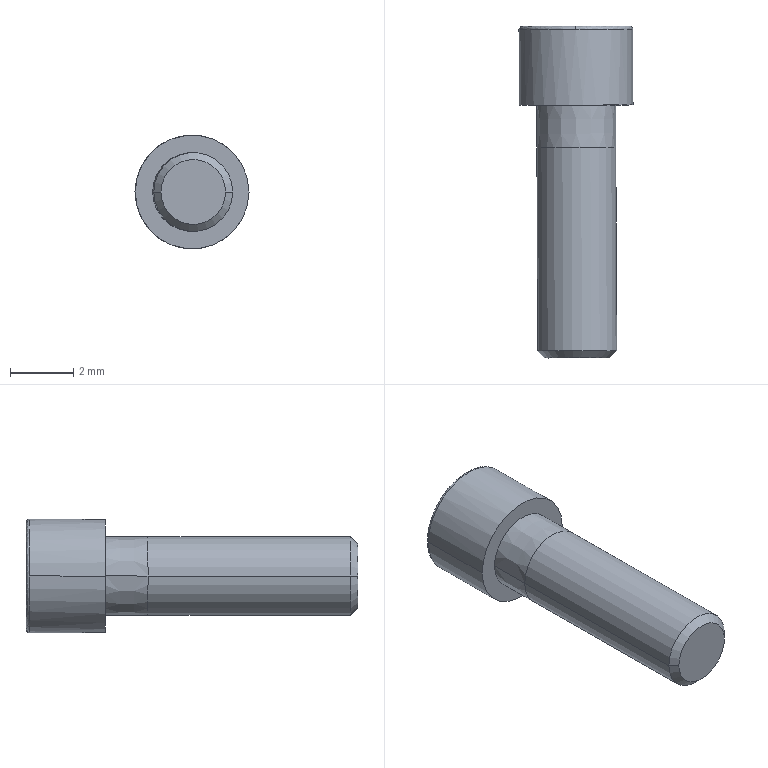Part | SolidWorks | features BaseBody 1 | 1 solid | 20 faces | box 3.61 x 10.512 x 3.6 mm | volume 60.691 mm3 | plane 10 | cylinder 4 | cone 4 | spline 2 | commonest cylinder face diameters 2.5 x2 3.6 x2
STEP:
#1=CARTESIAN_POINT('',(590.444,59.349,88.732));
#2=VERTEX_POINT('',#1);
#3=CARTESIAN_POINT('',(590.444,59.349,92.132));
#4=VERTEX_POINT('',#3);
#5=CARTESIAN_POINT('',(590.444,59.349,88.732));
#6=CARTESIAN_POINT('',(593.844,59.364,88.732));
#7=CARTESIAN_POINT('',(593.844,59.364,92.132));
#8=CARTESIAN_POINT('',(590.444,59.349,92.132));
#9=(BOUNDED_CURVE()B_SPLINE_CURVE(3,(#5,#6,#7,#8),.UNSPECIFIED.,.F.,.F.)B_SPLINE_CURVE_WITH_KNOTS((4,4),(0.,1.),.UNSPECIFIED.)CURVE()GEOMETRIC_REPRESENTATION_ITEM()RATIONAL_B_SPLINE_CURVE((1.,0.3333,0.3333,1.))REPRESENTATION_ITEM(''));
#10=EDGE_CURVE('',#2,#4,#9,.T.);
#11=ORIENTED_EDGE('',*,*,#10,.T.);
#12=CARTESIAN_POINT('',(590.444,59.249,92.232));
#13=VERTEX_POINT('',#12);
#14=CARTESIAN_POINT('',(590.444,59.249,92.132));
#15=DIRECTION('',(1.,0.004352,0.));
#16=DIRECTION('',(0.,0.,1.));
#17=AXIS2_PLACEMENT_3D('',#14,#15,#16);
#18=CIRCLE('',#17,0.1);
#19=EDGE_CURVE('',#4,#13,#18,.T.);
#20=ORIENTED_EDGE('',*,*,#19,.T.);
#21=CARTESIAN_POINT('',(592.244,59.257,90.432));
#22=VERTEX_POINT('',#21);
#23=CARTESIAN_POINT('',(590.444,59.249,90.432));
#24=DIRECTION('',(0.004352,-1.,0.));
#25=DIRECTION('',(-1.,-0.004352,0.));
#26=AXIS2_PLACEMENT_3D('',#23,#24,#25);
#27=CIRCLE('',#26,1.8);
#28=EDGE_CURVE('',#22,#13,#27,.T.);
#29=ORIENTED_EDGE('',*,*,#28,.F.);
#30=CARTESIAN_POINT('',(590.444,59.249,88.632));
#31=VERTEX_POINT('',#30);
#32=CARTESIAN_POINT('',(590.444,59.249,90.432));
#33=DIRECTION('',(0.004352,-1.,0.));
#34=DIRECTION('',(-1.,-0.004352,0.));
#35=AXIS2_PLACEMENT_3D('',#32,#33,#34);
#36=CIRCLE('',#35,1.8);
#37=EDGE_CURVE('',#31,#22,#36,.T.);
#38=ORIENTED_EDGE('',*,*,#37,.F.);
#39=CARTESIAN_POINT('',(590.444,59.249,88.732));
#40=DIRECTION('',(-1.,-0.004352,0.));
#41=DIRECTION('',(0.,0.,-1.));
#42=AXIS2_PLACEMENT_3D('',#39,#40,#41);
#43=CIRCLE('',#42,0.1);
#44=EDGE_CURVE('',#2,#31,#43,.T.);
#45=ORIENTED_EDGE('',*,*,#44,.F.);
#46=EDGE_LOOP('',(#11,#20,#29,#38,#45));
#47=FACE_OUTER_BOUND('',#46,.T.);
#48=CARTESIAN_POINT('',(590.444,59.349,92.132));
#49=CARTESIAN_POINT('',(593.844,59.364,92.132));
#50=CARTESIAN_POINT('',(593.844,59.364,88.732));
#51=CARTESIAN_POINT('',(590.444,59.349,88.732));
#52=CARTESIAN_POINT('',(590.444,59.349,92.191));
#53=CARTESIAN_POINT('',(593.961,59.365,92.191));
#54=CARTESIAN_POINT('',(593.961,59.365,88.673));
#55=CARTESIAN_POINT('',(590.444,59.349,88.673));
#56=CARTESIAN_POINT('',(590.444,59.308,92.232));
#57=CARTESIAN_POINT('',(594.044,59.323,92.232));
#58=CARTESIAN_POINT('',(594.044,59.323,88.632));
#59=CARTESIAN_POINT('',(590.444,59.308,88.632));
#60=CARTESIAN_POINT('',(590.444,59.249,92.232));
#61=CARTESIAN_POINT('',(594.044,59.265,92.232));
#62=CARTESIAN_POINT('',(594.044,59.265,88.632));
#63=CARTESIAN_POINT('',(590.444,59.249,88.632));
#64=(BOUNDED_SURFACE()B_SPLINE_SURFACE(3,3,((#48,#49,#50,#51),(#52,#53,#54,#55),(#56,#57,#58,#59),(#60,#61,#62,#63)),.UNSPECIFIED.,.F.,.F.,.T.)B_SPLINE_SURFACE_WITH_KNOTS((4,4),(4,4),(0.,1.),(0.,1.),.UNSPECIFIED.)GEOMETRIC_REPRESENTATION_ITEM()RATIONAL_B_SPLINE_SURFACE(((1.,0.3333,0.3333,1.),(0.8047,0.2682,0.2682,0.8047),(0.8047,0.2682,0.2682,0.8047),(1.,0.3333,0.3333,1.)))REPRESENTATION_ITEM('')SURFACE());
#65=ADVANCED_FACE('',(#47),#64,.T.);
#66=CARTESIAN_POINT('',(589.238,49.069,90.432));
#67=VERTEX_POINT('',#66);
#68=CARTESIAN_POINT('',(591.738,49.08,90.432));
#69=VERTEX_POINT('',#68);
#70=CARTESIAN_POINT('',(590.488,49.074,90.432));
#71=DIRECTION('',(-0.004352,1.,0.));
#72=DIRECTION('',(-1.,-0.004352,0.));
#73=AXIS2_PLACEMENT_3D('',#70,#71,#72);
#74=CIRCLE('',#73,1.25);
#75=EDGE_CURVE('',#67,#69,#74,.T.);
#76=ORIENTED_EDGE('',*,*,#75,.T.);
#77=CARTESIAN_POINT('',(591.71,55.505,90.432));
#78=VERTEX_POINT('',#77);
#79=CARTESIAN_POINT('',(591.724,52.292,90.432));
#80=DIRECTION('',(-0.004352,1.,0.));
#81=VECTOR('',#80,1000.);
#82=LINE('',#79,#81);
#83=EDGE_CURVE('',#69,#78,#82,.T.);
#84=ORIENTED_EDGE('',*,*,#83,.T.);
#85=CARTESIAN_POINT('',(589.211,55.494,90.432));
#86=VERTEX_POINT('',#85);
#87=CARTESIAN_POINT('',(590.461,55.499,90.432));
#88=DIRECTION('',(0.004352,-1.,0.));
#89=DIRECTION('',(-1.,-0.004352,0.));
#90=AXIS2_PLACEMENT_3D('',#87,#88,#89);
#91=CIRCLE('',#90,1.25);
#92=EDGE_CURVE('',#78,#86,#91,.T.);
#93=ORIENTED_EDGE('',*,*,#92,.T.);
#94=CARTESIAN_POINT('',(589.224,52.281,90.432));
#95=DIRECTION('',(-0.004352,1.,0.));
#96=VECTOR('',#95,1000.);
#97=LINE('',#94,#96);
#98=EDGE_CURVE('',#67,#86,#97,.T.);
#99=ORIENTED_EDGE('',*,*,#98,.F.);
#100=EDGE_LOOP('',(#76,#84,#93,#99));
#101=FACE_OUTER_BOUND('',#100,.T.);
#102=CARTESIAN_POINT('',(590.474,52.287,90.432));
#103=DIRECTION('',(-0.004352,1.,0.));
#104=DIRECTION('',(-1.,-0.004352,0.));
#105=AXIS2_PLACEMENT_3D('',#102,#103,#104);
#106=CYLINDRICAL_SURFACE('',#105,1.25);
#107=ADVANCED_FACE('',(#101),#106,.T.);
#108=CARTESIAN_POINT('',(591.704,56.855,90.432));
#109=VERTEX_POINT('',#108);
#110=CARTESIAN_POINT('',(589.205,56.844,90.432));
#111=VERTEX_POINT('',#110);
#112=CARTESIAN_POINT('',(590.455,56.849,90.432));
#113=DIRECTION('',(0.004352,-1.,0.));
#114=DIRECTION('',(1.,0.004352,0.));
#115=AXIS2_PLACEMENT_3D('',#112,#113,#114);
#116=CIRCLE('',#115,1.249);
#117=EDGE_CURVE('',#109,#111,#116,.T.);
#118=ORIENTED_EDGE('',*,*,#117,.T.);
#119=CARTESIAN_POINT('',(589.211,55.494,90.432));
#120=DIRECTION('',(0.003889,-1.,0.));
#121=VECTOR('',#120,1000.);
#122=LINE('',#119,#121);
#123=EDGE_CURVE('',#111,#86,#122,.T.);
#124=ORIENTED_EDGE('',*,*,#123,.T.);
#125=ORIENTED_EDGE('',*,*,#92,.F.);
#126=CARTESIAN_POINT('',(591.71,55.505,90.432));
#127=DIRECTION('',(0.004815,-1.,0.));
#128=VECTOR('',#127,1000.);
#129=LINE('',#126,#128);
#130=EDGE_CURVE('',#109,#78,#129,.T.);
#131=ORIENTED_EDGE('',*,*,#130,.F.);
#132=EDGE_LOOP('',(#118,#124,#125,#131));
#133=FACE_OUTER_BOUND('',#132,.T.);
#134=CARTESIAN_POINT('',(590.461,55.499,90.432));
#135=DIRECTION('',(0.004352,-1.,0.));
#136=DIRECTION('',(1.,0.004352,0.));
#137=AXIS2_PLACEMENT_3D('',#134,#135,#136);
#138=CONICAL_SURFACE('',#137,1.25,0.000463);
#139=ADVANCED_FACE('',(#133),#138,.T.);
#140=CARTESIAN_POINT('',(589.464,48.845,90.432));
#141=VERTEX_POINT('',#140);
#142=CARTESIAN_POINT('',(591.514,48.854,90.432));
#143=VERTEX_POINT('',#142);
#144=CARTESIAN_POINT('',(590.489,48.849,90.432));
#145=DIRECTION('',(-0.004352,1.,0.));
#146=DIRECTION('',(-1.,-0.004352,0.));
#147=AXIS2_PLACEMENT_3D('',#144,#145,#146);
#148=CIRCLE('',#147,1.025);
#149=EDGE_CURVE('',#141,#143,#148,.T.);
#150=ORIENTED_EDGE('',*,*,#149,.T.);
#151=CARTESIAN_POINT('',(591.738,49.08,90.432));
#152=DIRECTION('',(0.704,0.7102,0.));
#153=VECTOR('',#152,1000.);
#154=LINE('',#151,#153);
#155=EDGE_CURVE('',#143,#69,#154,.T.);
#156=ORIENTED_EDGE('',*,*,#155,.T.);
#157=ORIENTED_EDGE('',*,*,#75,.F.);
#158=CARTESIAN_POINT('',(589.238,49.069,90.432));
#159=DIRECTION('',(-0.7102,0.704,0.));
#160=VECTOR('',#159,1000.);
#161=LINE('',#158,#160);
#162=EDGE_CURVE('',#141,#67,#161,.T.);
#163=ORIENTED_EDGE('',*,*,#162,.F.);
#164=EDGE_LOOP('',(#150,#156,#157,#163));
#165=FACE_OUTER_BOUND('',#164,.T.);
#166=CARTESIAN_POINT('',(590.488,49.074,90.432));
#167=DIRECTION('',(-0.004352,1.,0.));
#168=DIRECTION('',(-1.,-0.004352,0.));
#169=AXIS2_PLACEMENT_3D('',#166,#167,#168);
#170=CONICAL_SURFACE('',#169,1.25,0.7854);
#171=ADVANCED_FACE('',(#165),#170,.T.);
#172=CARTESIAN_POINT('',(592.255,56.857,90.432));
#173=VERTEX_POINT('',#172);
#174=CARTESIAN_POINT('',(588.655,56.841,90.432));
#175=VERTEX_POINT('',#174);
#176=CARTESIAN_POINT('',(590.455,56.849,90.432));
#177=DIRECTION('',(0.004352,-1.,0.));
#178=DIRECTION('',(-1.,-0.004352,0.));
#179=AXIS2_PLACEMENT_3D('',#176,#177,#178);
#180=CIRCLE('',#179,1.8);
#181=EDGE_CURVE('',#173,#175,#180,.T.);
#182=ORIENTED_EDGE('',*,*,#181,.F.);
#183=CARTESIAN_POINT('',(592.249,58.057,90.432));
#184=DIRECTION('',(-0.004352,1.,0.));
#185=VECTOR('',#184,1000.);
#186=LINE('',#183,#185);
#187=EDGE_CURVE('',#173,#22,#186,.T.);
#188=ORIENTED_EDGE('',*,*,#187,.T.);
#189=ORIENTED_EDGE('',*,*,#28,.T.);
#190=CARTESIAN_POINT('',(588.644,59.241,90.432));
#191=VERTEX_POINT('',#190);
#192=CARTESIAN_POINT('',(590.444,59.249,90.432));
#193=DIRECTION('',(0.004352,-1.,0.));
#194=DIRECTION('',(-1.,-0.004352,0.));
#195=AXIS2_PLACEMENT_3D('',#192,#193,#194);
#196=CIRCLE('',#195,1.8);
#197=EDGE_CURVE('',#13,#191,#196,.T.);
#198=ORIENTED_EDGE('',*,*,#197,.T.);
#199=CARTESIAN_POINT('',(588.649,58.041,90.432));
#200=DIRECTION('',(-0.004352,1.,0.));
#201=VECTOR('',#200,1000.);
#202=LINE('',#199,#201);
#203=EDGE_CURVE('',#175,#191,#202,.T.);
#204=ORIENTED_EDGE('',*,*,#203,.F.);
#205=EDGE_LOOP('',(#182,#188,#189,#198,#204));
#206=FACE_OUTER_BOUND('',#205,.T.);
#207=CARTESIAN_POINT('',(590.449,58.049,90.432));
#208=DIRECTION('',(-0.004352,1.,0.));
#209=DIRECTION('',(-1.,-0.004352,0.));
#210=AXIS2_PLACEMENT_3D('',#207,#208,#209);
#211=CYLINDRICAL_SURFACE('',#210,1.8);
#212=ADVANCED_FACE('',(#206),#211,.T.);
#213=ORIENTED_EDGE('',*,*,#83,.F.);
#214=CARTESIAN_POINT('',(590.488,49.074,90.432));
#215=DIRECTION('',(-0.004352,1.,0.));
#216=DIRECTION('',(-1.,-0.004352,0.));
#217=AXIS2_PLACEMENT_3D('',#214,#215,#216);
#218=CIRCLE('',#217,1.25);
#219=EDGE_CURVE('',#69,#67,#218,.T.);
#220=ORIENTED_EDGE('',*,*,#219,.T.);
#221=ORIENTED_EDGE('',*,*,#98,.T.);
#222=CARTESIAN_POINT('',(590.461,55.499,90.432));
#223=DIRECTION('',(0.004352,-1.,0.));
#224=DIRECTION('',(-1.,-0.004352,0.));
#225=AXIS2_PLACEMENT_3D('',#222,#223,#224);
#226=CIRCLE('',#225,1.25);
#227=EDGE_CURVE('',#86,#78,#226,.T.);
#228=ORIENTED_EDGE('',*,*,#227,.T.);
#229=EDGE_LOOP('',(#213,#220,#221,#228));
#230=FACE_OUTER_BOUND('',#229,.T.);
#231=CARTESIAN_POINT('',(590.474,52.287,90.432));
#232=DIRECTION('',(-0.004352,1.,0.));
#233=DIRECTION('',(-1.,-0.004352,0.));
#234=AXIS2_PLACEMENT_3D('',#231,#232,#233);
#235=CYLINDRICAL_SURFACE('',#234,1.25);
#236=ADVANCED_FACE('',(#230),#235,.T.);
#237=ORIENTED_EDGE('',*,*,#123,.F.);
#238=CARTESIAN_POINT('',(590.455,56.849,90.432));
#239=DIRECTION('',(0.004352,-1.,0.));
#240=DIRECTION('',(1.,0.004352,0.));
#241=AXIS2_PLACEMENT_3D('',#238,#239,#240);
#242=CIRCLE('',#241,1.249);
#243=EDGE_CURVE('',#111,#109,#242,.T.);
#244=ORIENTED_EDGE('',*,*,#243,.T.);
#245=ORIENTED_EDGE('',*,*,#130,.T.);
#246=ORIENTED_EDGE('',*,*,#227,.F.);
#247=EDGE_LOOP('',(#237,#244,#245,#246));
#248=FACE_OUTER_BOUND('',#247,.T.);
#249=CARTESIAN_POINT('',(590.461,55.499,90.432));
#250=DIRECTION('',(0.004352,-1.,0.));
#251=DIRECTION('',(1.,0.004352,0.));
#252=AXIS2_PLACEMENT_3D('',#249,#250,#251);
#253=CONICAL_SURFACE('',#252,1.25,0.000463);
#254=ADVANCED_FACE('',(#248),#253,.T.);
#255=ORIENTED_EDGE('',*,*,#155,.F.);
#256=CARTESIAN_POINT('',(590.489,48.849,90.432));
#257=DIRECTION('',(-0.004352,1.,0.));
#258=DIRECTION('',(-1.,-0.004352,0.));
#259=AXIS2_PLACEMENT_3D('',#256,#257,#258);
#260=CIRCLE('',#259,1.025);
#261=EDGE_CURVE('',#143,#141,#260,.T.);
#262=ORIENTED_EDGE('',*,*,#261,.T.);
#263=ORIENTED_EDGE('',*,*,#162,.T.);
#264=ORIENTED_EDGE('',*,*,#219,.F.);
#265=EDGE_LOOP('',(#255,#262,#263,#264));
#266=FACE_OUTER_BOUND('',#265,.T.);
#267=CARTESIAN_POINT('',(590.488,49.074,90.432));
#268=DIRECTION('',(-0.004352,1.,0.));
#269=DIRECTION('',(-1.,-0.004352,0.));
#270=AXIS2_PLACEMENT_3D('',#267,#268,#269);
#271=CONICAL_SURFACE('',#270,1.25,0.7854);
#272=ADVANCED_FACE('',(#266),#271,.T.);
#273=ORIENTED_EDGE('',*,*,#117,.F.);
#274=ORIENTED_EDGE('',*,*,#243,.F.);
#275=EDGE_LOOP('',(#273,#274));
#276=FACE_BOUND('',#275,.T.);
#277=CARTESIAN_POINT('',(590.455,56.849,90.432));
#278=DIRECTION('',(0.004352,-1.,0.));
#279=DIRECTION('',(-1.,-0.004352,0.));
#280=AXIS2_PLACEMENT_3D('',#277,#278,#279);
#281=CIRCLE('',#280,1.8);
#282=EDGE_CURVE('',#175,#173,#281,.T.);
#283=ORIENTED_EDGE('',*,*,#282,.T.);
#284=ORIENTED_EDGE('',*,*,#181,.T.);
#285=EDGE_LOOP('',(#283,#284));
#286=FACE_OUTER_BOUND('',#285,.T.);
#287=CARTESIAN_POINT('',(590.455,56.849,89.532));
#288=DIRECTION('',(0.004352,-1.,0.));
#289=DIRECTION('',(1.,0.004352,0.));
#290=AXIS2_PLACEMENT_3D('',#287,#288,#289);
#291=PLANE('',#290);
#292=ADVANCED_FACE('',(#276,#286),#291,.T.);
#293=ORIENTED_EDGE('',*,*,#149,.F.);
#294=ORIENTED_EDGE('',*,*,#261,.F.);
#295=EDGE_LOOP('',(#293,#294));
#296=FACE_OUTER_BOUND('',#295,.T.);
#297=CARTESIAN_POINT('',(590.489,48.849,89.919));
#298=DIRECTION('',(0.004352,-1.,0.));
#299=DIRECTION('',(1.,0.004352,0.));
#300=AXIS2_PLACEMENT_3D('',#297,#298,#299);
#301=PLANE('',#300);
#302=ADVANCED_FACE('',(#296),#301,.T.);
#303=ORIENTED_EDGE('',*,*,#187,.F.);
#304=ORIENTED_EDGE('',*,*,#282,.F.);
#305=ORIENTED_EDGE('',*,*,#203,.T.);
#306=CARTESIAN_POINT('',(590.444,59.249,90.432));
#307=DIRECTION('',(0.004352,-1.,0.));
#308=DIRECTION('',(-1.,-0.004352,0.));
#309=AXIS2_PLACEMENT_3D('',#306,#307,#308);
#310=CIRCLE('',#309,1.8);
#311=EDGE_CURVE('',#191,#31,#310,.T.);
#312=ORIENTED_EDGE('',*,*,#311,.T.);
#313=ORIENTED_EDGE('',*,*,#37,.T.);
#314=EDGE_LOOP('',(#303,#304,#305,#312,#313));
#315=FACE_OUTER_BOUND('',#314,.T.);
#316=CARTESIAN_POINT('',(590.449,58.049,90.432));
#317=DIRECTION('',(-0.004352,1.,0.));
#318=DIRECTION('',(-1.,-0.004352,0.));
#319=AXIS2_PLACEMENT_3D('',#316,#317,#318);
#320=CYLINDRICAL_SURFACE('',#319,1.8);
#321=ADVANCED_FACE('',(#315),#320,.T.);
#322=ORIENTED_EDGE('',*,*,#19,.F.);
#323=CARTESIAN_POINT('',(590.444,59.349,92.132));
#324=CARTESIAN_POINT('',(587.044,59.334,92.132));
#325=CARTESIAN_POINT('',(587.044,59.334,88.732));
#326=CARTESIAN_POINT('',(590.444,59.349,88.732));
#327=(BOUNDED_CURVE()B_SPLINE_CURVE(3,(#323,#324,#325,#326),.UNSPECIFIED.,.F.,.T.)B_SPLINE_CURVE_WITH_KNOTS((4,4),(0.,1.),.UNSPECIFIED.)CURVE()GEOMETRIC_REPRESENTATION_ITEM()RATIONAL_B_SPLINE_CURVE((1.,0.3333,0.3333,1.))REPRESENTATION_ITEM(''));
#328=EDGE_CURVE('',#4,#2,#327,.T.);
#329=ORIENTED_EDGE('',*,*,#328,.T.);
#330=ORIENTED_EDGE('',*,*,#44,.T.);
#331=ORIENTED_EDGE('',*,*,#311,.F.);
#332=ORIENTED_EDGE('',*,*,#197,.F.);
#333=EDGE_LOOP('',(#322,#329,#330,#331,#332));
#334=FACE_OUTER_BOUND('',#333,.T.);
#335=CARTESIAN_POINT('',(590.444,59.349,88.732));
#336=CARTESIAN_POINT('',(587.044,59.334,88.732));
#337=CARTESIAN_POINT('',(587.044,59.334,92.132));
#338=CARTESIAN_POINT('',(590.444,59.349,92.132));
#339=CARTESIAN_POINT('',(590.444,59.349,88.673));
#340=CARTESIAN_POINT('',(586.927,59.334,88.673));
#341=CARTESIAN_POINT('',(586.927,59.334,92.191));
#342=CARTESIAN_POINT('',(590.444,59.349,92.191));
#343=CARTESIAN_POINT('',(590.444,59.308,88.632));
#344=CARTESIAN_POINT('',(586.844,59.292,88.632));
#345=CARTESIAN_POINT('',(586.844,59.292,92.232));
#346=CARTESIAN_POINT('',(590.444,59.308,92.232));
#347=CARTESIAN_POINT('',(590.444,59.249,88.632));
#348=CARTESIAN_POINT('',(586.844,59.234,88.632));
#349=CARTESIAN_POINT('',(586.844,59.234,92.232));
#350=CARTESIAN_POINT('',(590.444,59.249,92.232));
#351=(BOUNDED_SURFACE()B_SPLINE_SURFACE(3,3,((#335,#336,#337,#338),(#339,#340,#341,#342),(#343,#344,#345,#346),(#347,#348,#349,#350)),.UNSPECIFIED.,.F.,.F.,.T.)B_SPLINE_SURFACE_WITH_KNOTS((4,4),(4,4),(0.,1.),(0.,1.),.UNSPECIFIED.)GEOMETRIC_REPRESENTATION_ITEM()RATIONAL_B_SPLINE_SURFACE(((1.,0.3333,0.3333,1.),(0.8047,0.2682,0.2682,0.8047),(0.8047,0.2682,0.2682,0.8047),(1.,0.3333,0.3333,1.)))REPRESENTATION_ITEM('')SURFACE());
#352=ADVANCED_FACE('',(#334),#351,.T.);
#353=ORIENTED_EDGE('',*,*,#328,.F.);
#354=ORIENTED_EDGE('',*,*,#10,.F.);
#355=EDGE_LOOP('',(#353,#354));
#356=FACE_OUTER_BOUND('',#355,.T.);
#357=CARTESIAN_POINT('',(591.444,59.354,91.009));
#358=VERTEX_POINT('',#357);
#359=CARTESIAN_POINT('',(590.444,59.349,91.587));
#360=VERTEX_POINT('',#359);
#361=CARTESIAN_POINT('',(591.444,59.354,91.009));
#362=DIRECTION('',(-0.866,-0.003769,0.5));
#363=VECTOR('',#362,1000.);
#364=LINE('',#361,#363);
#365=EDGE_CURVE('',#358,#360,#364,.T.);
#366=ORIENTED_EDGE('',*,*,#365,.T.);
#367=CARTESIAN_POINT('',(589.444,59.345,91.009));
#368=VERTEX_POINT('',#367);
#369=CARTESIAN_POINT('',(590.444,59.349,91.587));
#370=DIRECTION('',(-0.866,-0.003769,-0.5));
#371=VECTOR('',#370,1000.);
#372=LINE('',#369,#371);
#373=EDGE_CURVE('',#360,#368,#372,.T.);
#374=ORIENTED_EDGE('',*,*,#373,.T.);
#375=CARTESIAN_POINT('',(589.444,59.345,89.855));
#376=VERTEX_POINT('',#375);
#377=CARTESIAN_POINT('',(589.444,59.345,89.582));
#378=DIRECTION('',(0.,0.,-1.));
#379=VECTOR('',#378,1000.);
#380=LINE('',#377,#379);
#381=EDGE_CURVE('',#368,#376,#380,.T.);
#382=ORIENTED_EDGE('',*,*,#381,.T.);
#383=CARTESIAN_POINT('',(590.444,59.349,89.277));
#384=VERTEX_POINT('',#383);
#385=CARTESIAN_POINT('',(589.444,59.345,89.855));
#386=DIRECTION('',(0.866,0.003769,-0.5));
#387=VECTOR('',#386,1000.);
#388=LINE('',#385,#387);
#389=EDGE_CURVE('',#376,#384,#388,.T.);
#390=ORIENTED_EDGE('',*,*,#389,.T.);
#391=CARTESIAN_POINT('',(591.444,59.354,89.855));
#392=VERTEX_POINT('',#391);
#393=CARTESIAN_POINT('',(590.444,59.349,89.277));
#394=DIRECTION('',(0.866,0.003769,0.5));
#395=VECTOR('',#394,1000.);
#396=LINE('',#393,#395);
#397=EDGE_CURVE('',#384,#392,#396,.T.);
#398=ORIENTED_EDGE('',*,*,#397,.T.);
#399=CARTESIAN_POINT('',(591.444,59.354,89.582));
#400=DIRECTION('',(0.,0.,1.));
#401=VECTOR('',#400,1000.);
#402=LINE('',#399,#401);
#403=EDGE_CURVE('',#392,#358,#402,.T.);
#404=ORIENTED_EDGE('',*,*,#403,.T.);
#405=EDGE_LOOP('',(#366,#374,#382,#390,#398,#404));
#406=FACE_BOUND('',#405,.T.);
#407=CARTESIAN_POINT('',(590.444,59.349,89.582));
#408=DIRECTION('',(-0.004352,1.,0.));
#409=DIRECTION('',(-1.,-0.004352,0.));
#410=AXIS2_PLACEMENT_3D('',#407,#408,#409);
#411=PLANE('',#410);
#412=ADVANCED_FACE('',(#356,#406),#411,.T.);
#413=CARTESIAN_POINT('',(589.449,58.245,91.009));
#414=VERTEX_POINT('',#413);
#415=CARTESIAN_POINT('',(589.444,59.345,91.009));
#416=DIRECTION('',(0.004352,-1.,0.));
#417=VECTOR('',#416,1000.);
#418=LINE('',#415,#417);
#419=EDGE_CURVE('',#368,#414,#418,.T.);
#420=ORIENTED_EDGE('',*,*,#419,.F.);
#421=ORIENTED_EDGE('',*,*,#373,.F.);
#422=CARTESIAN_POINT('',(590.449,58.249,91.587));
#423=VERTEX_POINT('',#422);
#424=CARTESIAN_POINT('',(590.449,58.249,91.587));
#425=DIRECTION('',(-0.004352,1.,0.));
#426=VECTOR('',#425,1000.);
#427=LINE('',#424,#426);
#428=EDGE_CURVE('',#423,#360,#427,.T.);
#429=ORIENTED_EDGE('',*,*,#428,.F.);
#430=CARTESIAN_POINT('',(589.449,58.245,91.009));
#431=DIRECTION('',(0.866,0.003769,0.5));
#432=VECTOR('',#431,1000.);
#433=LINE('',#430,#432);
#434=EDGE_CURVE('',#414,#423,#433,.T.);
#435=ORIENTED_EDGE('',*,*,#434,.F.);
#436=EDGE_LOOP('',(#420,#421,#429,#435));
#437=FACE_OUTER_BOUND('',#436,.T.);
#438=CARTESIAN_POINT('',(589.444,59.345,91.009));
#439=DIRECTION('',(-0.5,-0.002176,0.866));
#440=DIRECTION('',(0.866,0.,0.5));
#441=AXIS2_PLACEMENT_3D('',#438,#439,#440);
#442=PLANE('',#441);
#443=ADVANCED_FACE('',(#437),#442,.F.);
#444=ORIENTED_EDGE('',*,*,#428,.T.);
#445=ORIENTED_EDGE('',*,*,#365,.F.);
#446=CARTESIAN_POINT('',(591.449,58.254,91.009));
#447=VERTEX_POINT('',#446);
#448=CARTESIAN_POINT('',(591.449,58.254,91.009));
#449=DIRECTION('',(-0.004352,1.,0.));
#450=VECTOR('',#449,1000.);
#451=LINE('',#448,#450);
#452=EDGE_CURVE('',#447,#358,#451,.T.);
#453=ORIENTED_EDGE('',*,*,#452,.F.);
#454=CARTESIAN_POINT('',(590.449,58.249,91.587));
#455=DIRECTION('',(0.866,0.003769,-0.5));
#456=VECTOR('',#455,1000.);
#457=LINE('',#454,#456);
#458=EDGE_CURVE('',#423,#447,#457,.T.);
#459=ORIENTED_EDGE('',*,*,#458,.F.);
#460=EDGE_LOOP('',(#444,#445,#453,#459));
#461=FACE_OUTER_BOUND('',#460,.T.);
#462=CARTESIAN_POINT('',(590.444,59.349,91.587));
#463=DIRECTION('',(0.5,0.002176,0.866));
#464=DIRECTION('',(0.866,0.,-0.5));
#465=AXIS2_PLACEMENT_3D('',#462,#463,#464);
#466=PLANE('',#465);
#467=ADVANCED_FACE('',(#461),#466,.F.);
#468=ORIENTED_EDGE('',*,*,#452,.T.);
#469=ORIENTED_EDGE('',*,*,#403,.F.);
#470=CARTESIAN_POINT('',(591.449,58.254,89.855));
#471=VERTEX_POINT('',#470);
#472=CARTESIAN_POINT('',(591.444,59.354,89.855));
#473=DIRECTION('',(-0.004352,1.,0.));
#474=VECTOR('',#473,1000.);
#475=LINE('',#472,#474);
#476=EDGE_CURVE('',#471,#392,#475,.T.);
#477=ORIENTED_EDGE('',*,*,#476,.F.);
#478=CARTESIAN_POINT('',(591.449,58.254,91.009));
#479=DIRECTION('',(0.,0.,-1.));
#480=VECTOR('',#479,1000.);
#481=LINE('',#478,#480);
#482=EDGE_CURVE('',#447,#471,#481,.T.);
#483=ORIENTED_EDGE('',*,*,#482,.F.);
#484=EDGE_LOOP('',(#468,#469,#477,#483));
#485=FACE_OUTER_BOUND('',#484,.T.);
#486=CARTESIAN_POINT('',(591.444,59.354,91.009));
#487=DIRECTION('',(1.,0.004352,0.));
#488=DIRECTION('',(-0.004352,1.,0.));
#489=AXIS2_PLACEMENT_3D('',#486,#487,#488);
#490=PLANE('',#489);
#491=ADVANCED_FACE('',(#485),#490,.F.);
#492=ORIENTED_EDGE('',*,*,#476,.T.);
#493=ORIENTED_EDGE('',*,*,#397,.F.);
#494=CARTESIAN_POINT('',(590.449,58.249,89.277));
#495=VERTEX_POINT('',#494);
#496=CARTESIAN_POINT('',(590.449,58.249,89.277));
#497=DIRECTION('',(-0.004352,1.,0.));
#498=VECTOR('',#497,1000.);
#499=LINE('',#496,#498);
#500=EDGE_CURVE('',#495,#384,#499,.T.);
#501=ORIENTED_EDGE('',*,*,#500,.F.);
#502=CARTESIAN_POINT('',(591.449,58.254,89.855));
#503=DIRECTION('',(-0.866,-0.003769,-0.5));
#504=VECTOR('',#503,1000.);
#505=LINE('',#502,#504);
#506=EDGE_CURVE('',#471,#495,#505,.T.);
#507=ORIENTED_EDGE('',*,*,#506,.F.);
#508=EDGE_LOOP('',(#492,#493,#501,#507));
#509=FACE_OUTER_BOUND('',#508,.T.);
#510=CARTESIAN_POINT('',(591.444,59.354,89.855));
#511=DIRECTION('',(0.5,0.002176,-0.866));
#512=DIRECTION('',(-0.866,0.,-0.5));
#513=AXIS2_PLACEMENT_3D('',#510,#511,#512);
#514=PLANE('',#513);
#515=ADVANCED_FACE('',(#509),#514,.F.);
#516=ORIENTED_EDGE('',*,*,#500,.T.);
#517=ORIENTED_EDGE('',*,*,#389,.F.);
#518=CARTESIAN_POINT('',(589.449,58.245,89.855));
#519=VERTEX_POINT('',#518);
#520=CARTESIAN_POINT('',(589.449,58.245,89.855));
#521=DIRECTION('',(-0.004352,1.,0.));
#522=VECTOR('',#521,1000.);
#523=LINE('',#520,#522);
#524=EDGE_CURVE('',#519,#376,#523,.T.);
#525=ORIENTED_EDGE('',*,*,#524,.F.);
#526=CARTESIAN_POINT('',(590.449,58.249,89.277));
#527=DIRECTION('',(-0.866,-0.003769,0.5));
#528=VECTOR('',#527,1000.);
#529=LINE('',#526,#528);
#530=EDGE_CURVE('',#495,#519,#529,.T.);
#531=ORIENTED_EDGE('',*,*,#530,.F.);
#532=EDGE_LOOP('',(#516,#517,#525,#531));
#533=FACE_OUTER_BOUND('',#532,.T.);
#534=CARTESIAN_POINT('',(590.444,59.349,89.277));
#535=DIRECTION('',(-0.5,-0.002176,-0.866));
#536=DIRECTION('',(-0.866,0.,0.5));
#537=AXIS2_PLACEMENT_3D('',#534,#535,#536);
#538=PLANE('',#537);
#539=ADVANCED_FACE('',(#533),#538,.F.);
#540=ORIENTED_EDGE('',*,*,#524,.T.);
#541=ORIENTED_EDGE('',*,*,#381,.F.);
#542=ORIENTED_EDGE('',*,*,#419,.T.);
#543=CARTESIAN_POINT('',(589.449,58.245,89.855));
#544=DIRECTION('',(0.,0.,1.));
#545=VECTOR('',#544,1000.);
#546=LINE('',#543,#545);
#547=EDGE_CURVE('',#519,#414,#546,.T.);
#548=ORIENTED_EDGE('',*,*,#547,.F.);
#549=EDGE_LOOP('',(#540,#541,#542,#548));
#550=FACE_OUTER_BOUND('',#549,.T.);
#551=CARTESIAN_POINT('',(589.444,59.345,89.855));
#552=DIRECTION('',(-1.,-0.004352,0.));
#553=DIRECTION('',(0.004352,-1.,0.));
#554=AXIS2_PLACEMENT_3D('',#551,#552,#553);
#555=PLANE('',#554);
#556=ADVANCED_FACE('',(#550),#555,.F.);
#557=ORIENTED_EDGE('',*,*,#506,.T.);
#558=ORIENTED_EDGE('',*,*,#530,.T.);
#559=ORIENTED_EDGE('',*,*,#547,.T.);
#560=ORIENTED_EDGE('',*,*,#434,.T.);
#561=ORIENTED_EDGE('',*,*,#458,.T.);
#562=ORIENTED_EDGE('',*,*,#482,.T.);
#563=EDGE_LOOP('',(#557,#558,#559,#560,#561,#562));
#564=FACE_OUTER_BOUND('',#563,.T.);
#565=CARTESIAN_POINT('',(590.449,58.249,90.432));
#566=DIRECTION('',(-0.004352,1.,0.));
#567=DIRECTION('',(-1.,-0.004352,0.));
#568=AXIS2_PLACEMENT_3D('',#565,#566,#567);
#569=PLANE('',#568);
#570=ADVANCED_FACE('',(#564),#569,.T.);
#571=CLOSED_SHELL('',(#65,#107,#139,#171,#212,#236,#254,#272,#292,#302,#321,#352,#412,#443,#467,#491,#515,#539,#556,#570));
#572=MANIFOLD_SOLID_BREP('',#571);
#573=CARTESIAN_POINT('',(0.,0.,0.));
#574=DIRECTION('',(0.,0.,1.));
#575=DIRECTION('',(1.,0.,0.));
#576=AXIS2_PLACEMENT_3D('',#573,#574,#575);
#577=(LENGTH_UNIT()NAMED_UNIT(*)SI_UNIT(.MILLI.,.METRE.));
#578=UNCERTAINTY_MEASURE_WITH_UNIT(LENGTH_MEASURE(0.00001),#577,'','');
#579=(NAMED_UNIT(*)PLANE_ANGLE_UNIT()SI_UNIT($,.RADIAN.));
#580=(NAMED_UNIT(*)SI_UNIT($,.STERADIAN.)SOLID_ANGLE_UNIT());
#581=(GEOMETRIC_REPRESENTATION_CONTEXT(3)GLOBAL_UNCERTAINTY_ASSIGNED_CONTEXT((#578))GLOBAL_UNIT_ASSIGNED_CONTEXT((#577,#579,#580))REPRESENTATION_CONTEXT('',''));
#582=ADVANCED_BREP_SHAPE_REPRESENTATION('',(#572,#576),#581);